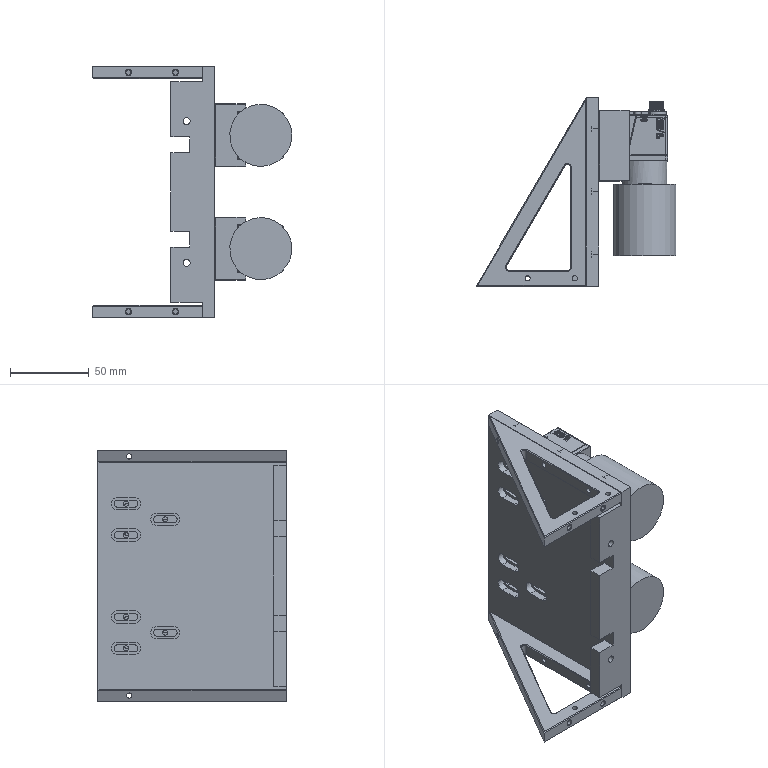Part | SolidWorks | 7 solids | 3226 faces | volume 428016 mm3 | plane 1742 | cylinder 896 | spline 342 | cone 240 | torus 6 | commonest cylinder face diameters 0.4 x168 1.4 x78 8.5 x42 2 x40 3.3 x40 8 x38